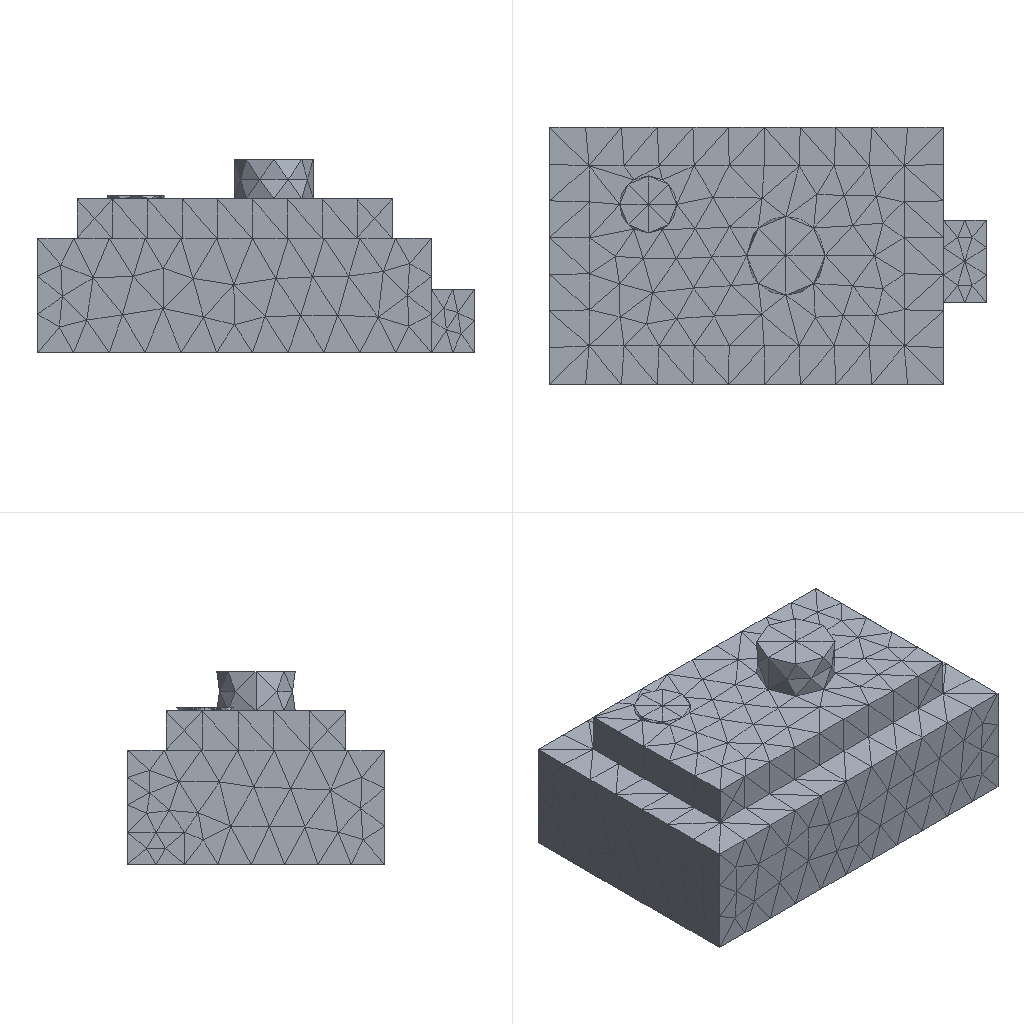Simulation study | ansys mapdl
Set-up summary:
category,name,step,type,value,unit,region
solver,ansys_mapdl
units,mm-N-s-tonne (MPa),,inferred,E=210000 density=
analysis,model,,static
mesh,nodes,,,4668
mesh,elements,,,2803
element_type,SOLID187,,,2803
material,mat 1,,E,210000
material,mat 1,,nu,0.3
load,,model,body load temp,,,all
load,,model,force,"1000 [dir=(0, 0, -1) n=92]",,node list
bc,,model,fixed,"[dofs=UX,UY,UZ n=5132]",,node list
Ansys APDL input file, long lists of numbers shortened:
/COM,ANSYS RELEASE 2026 R1           BUILD 26.1      UP20260202       09:11:24
/PREP7
/NOPR
/TITLE,2
ANTYPE, 0
*IF,_CDRDOFF,EQ,1,THEN     !if solid model was read in
_CDRDOFF=             !reset flag, numoffs already performed
*ELSE              !offset database for the following FE model
NUMOFF,NODE,     4668
NUMOFF,ELEM,     2803
NUMOFF,MAT ,        1
NUMOFF,TYPE,        1
*ENDIF
*SET,_RETURN ,  0.
*SET,_STATUS ,  0.
*SET,_UIQR   ,  92.
*SET,__FLOATPARAMETER__,  4668.
DOF,DELETE
ETBLOCK,        1,        1
(2i9,19a9)
        1      187        0        0        0        0        0        0        0        0        0        0        0        0        0        0        0        0        0        0        0
       -1
NBLOCK,6,SOLID,      4668,      4668
(3i9,6e21.13e3)
        1        0        0-3.9150000000000E+001 3.6000000000000E+001 9.0000000000000E+000
! (4667 more lines like these left out)
N,UNBL,LOC,       -1,
EBLOCK,19,SOLID,      2803,      2803
(19i10)
         1         1         1         1         0         0         0         0        10         0         1      1771      1772      1773      1774      2039      2040      2041      2042
! (5605 more lines like these left out)
        -1
MPTEMP,UNBL, 1, 1,  0.    ,
MPDATA,UNBL, 1,EX  ,       1, 1,  210000.000    ,
MPTEMP,UNBL, 1, 1,  0.    ,
MPDATA,UNBL, 1,NUXY,       1, 1, 0.3    ,
MPTEMP,UNBL, 1, 1,  0.    ,
MPDATA,UNBL, 1,PRXY,       1, 1, 0.3    ,
EXTOPT,ATTR,      0,      0,      0
EXTOPT,ESIZE,  0,  0.
EXTOPT,ACLEAR,      0
TREF,  0.
IRLF,  0
BFUNIF,TEMP,_TINY
ACEL,  0.    ,  0.    ,  0.
OMEGA,  0.    ,  0.    ,  0.
DOMEGA,  0.    ,  0.    ,  0.
CGLOC,  0.    ,  0.    ,  0.
CGOMEGA,  0.    ,  0.    ,  0.
DCGOMG,  0.    ,  0.    ,  0.
KUSE,     0
TIME,  0.
ALPHAD,  0.
BETAD,  0.
DMPRAT,  0.
DMPSTR,  0.
CRPLIM, 0.1    ,   0
CRPLIM,  0.    ,   1
NCNV,     0, 1.000000000E+12,     0,  0.    ,  0.
NEQIT,     0
ERESX,DEFA
DBLOCK,      5132
(i9,a6,2(pg16.9))
        1  UX    0.00000000      0.00000000
! (5131 more lines like these left out)
       -1
FBLOCK,        92
(i9,a6,2(pg16.9))
      870  FZ   -10.8695652      0.00000000
! (91 more lines like these left out)
       -1
/GO
FINISH
Results summary:
result,analysis_type_db,,,static,unstated
result,n_sets,,,1,unstated
result,load_steps[0].set,load_step=1,,1,unstated
result,load_steps[0].substep,load_step=1,,1,unstated
result,load_steps[0].time,load_step=1,,1,unstated
result,load_steps[0].freq,load_step=1,,1,unstated
result,load_steps[0].max_usum,load_step=1,,0.0003029,unstated
result,load_steps[0].max_seqv,load_step=1,,2.895,unstated
result,load_steps[0].reaction_sum.FX,load_step=1,,-4.13611e-12,unstated
result,load_steps[0].reaction_sum.FY,load_step=1,,-1.27529e-12,unstated
result,load_steps[0].reaction_sum.FZ,load_step=1,,1000,unstated
result,load_steps[0].reaction_sum.MX,load_step=1,,0,unstated
result,load_steps[0].reaction_sum.MY,load_step=1,,0,unstated
result,load_steps[0].reaction_sum.MZ,load_step=1,,0,unstated
result,convergence,,,results present for all listed sets,unstated